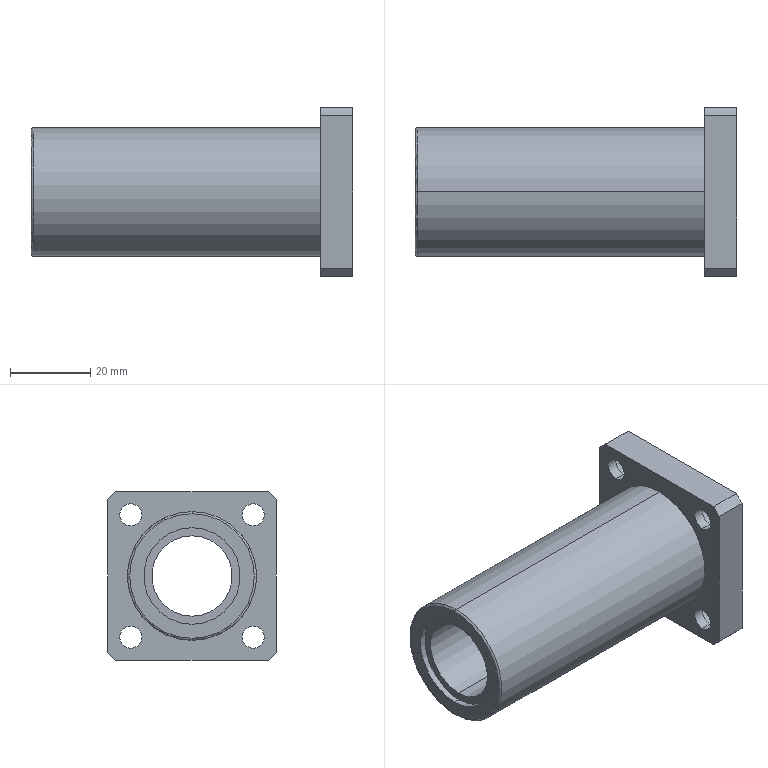Part | STEP file | LMK20LUU  | 1 solid | 43 faces | box 80 x 42 x 42 mm | volume 44458 mm3 | cylinder 24 | plane 17 | torus 2 | commonest cylinder face diameters 5.5 x8 10 x8 24 x4 20 x2 32 x2